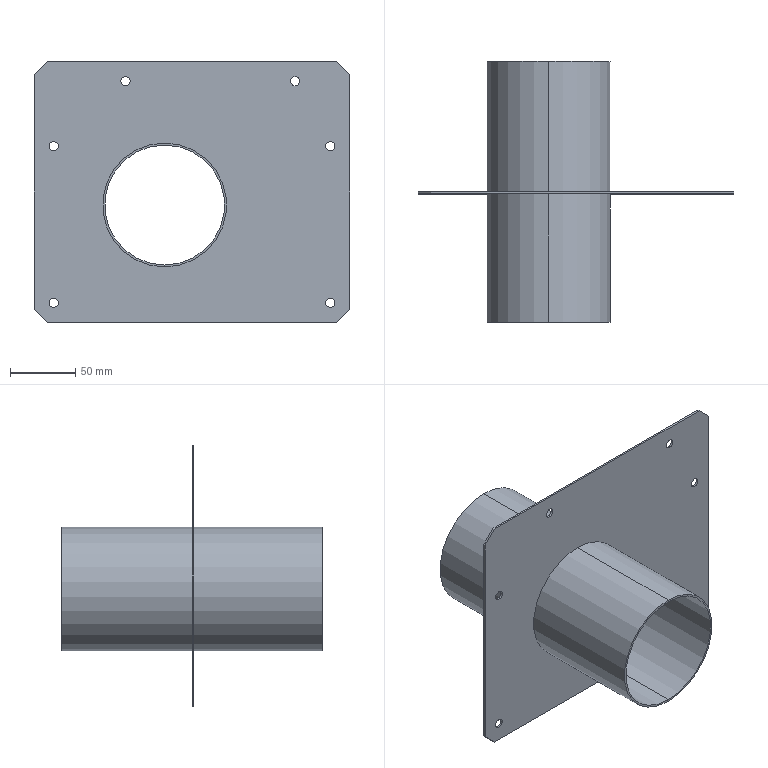Part | SolidWorks | features BaseBody 1 | 1 solid | 30 faces | box 242 x 200 x 200 mm | volume 149443 mm3 | cylinder 18 | plane 12 | commonest cylinder face diameters 7 x12 95 x4 92 x2
STEP:
#1=CARTESIAN_POINT('',(-51.,0.,88.5));
#2=VERTEX_POINT('',#1);
#3=CARTESIAN_POINT('',(-51.,0.,81.5));
#4=VERTEX_POINT('',#3);
#5=CARTESIAN_POINT('',(-51.,0.,85.));
#6=DIRECTION('',(0.,-1.,0.));
#7=DIRECTION('',(0.,0.,1.));
#8=AXIS2_PLACEMENT_3D('',#5,#6,#7);
#9=CIRCLE('',#8,3.5);
#10=EDGE_CURVE('',#2,#4,#9,.T.);
#11=ORIENTED_EDGE('',*,*,#10,.T.);
#12=CARTESIAN_POINT('',(-51.,1.5,81.5));
#13=VERTEX_POINT('',#12);
#14=CARTESIAN_POINT('',(-51.,-98.501,81.5));
#15=DIRECTION('',(0.,1.,0.));
#16=VECTOR('',#15,1000.);
#17=LINE('',#14,#16);
#18=EDGE_CURVE('',#4,#13,#17,.T.);
#19=ORIENTED_EDGE('',*,*,#18,.T.);
#20=CARTESIAN_POINT('',(-51.,1.5,88.5));
#21=VERTEX_POINT('',#20);
#22=CARTESIAN_POINT('',(-51.,1.5,85.));
#23=DIRECTION('',(0.,1.,0.));
#24=DIRECTION('',(0.,0.,1.));
#25=AXIS2_PLACEMENT_3D('',#22,#23,#24);
#26=CIRCLE('',#25,3.5);
#27=EDGE_CURVE('',#13,#21,#26,.T.);
#28=ORIENTED_EDGE('',*,*,#27,.T.);
#29=CARTESIAN_POINT('',(-51.,-98.501,88.5));
#30=DIRECTION('',(0.,1.,0.));
#31=VECTOR('',#30,1000.);
#32=LINE('',#29,#31);
#33=EDGE_CURVE('',#2,#21,#32,.T.);
#34=ORIENTED_EDGE('',*,*,#33,.F.);
#35=EDGE_LOOP('',(#11,#19,#28,#34));
#36=FACE_OUTER_BOUND('',#35,.T.);
#37=CARTESIAN_POINT('',(-51.,-98.501,85.));
#38=DIRECTION('',(0.,1.,0.));
#39=DIRECTION('',(0.,0.,1.));
#40=AXIS2_PLACEMENT_3D('',#37,#38,#39);
#41=CYLINDRICAL_SURFACE('',#40,3.5);
#42=ADVANCED_FACE('',(#36),#41,.F.);
#43=CARTESIAN_POINT('',(79.,0.,88.5));
#44=VERTEX_POINT('',#43);
#45=CARTESIAN_POINT('',(79.,0.,81.5));
#46=VERTEX_POINT('',#45);
#47=CARTESIAN_POINT('',(79.,0.,85.));
#48=DIRECTION('',(0.,-1.,0.));
#49=DIRECTION('',(0.,0.,1.));
#50=AXIS2_PLACEMENT_3D('',#47,#48,#49);
#51=CIRCLE('',#50,3.5);
#52=EDGE_CURVE('',#44,#46,#51,.T.);
#53=ORIENTED_EDGE('',*,*,#52,.T.);
#54=CARTESIAN_POINT('',(79.,1.5,81.5));
#55=VERTEX_POINT('',#54);
#56=CARTESIAN_POINT('',(79.,-98.501,81.5));
#57=DIRECTION('',(0.,1.,0.));
#58=VECTOR('',#57,1000.);
#59=LINE('',#56,#58);
#60=EDGE_CURVE('',#46,#55,#59,.T.);
#61=ORIENTED_EDGE('',*,*,#60,.T.);
#62=CARTESIAN_POINT('',(79.,1.5,88.5));
#63=VERTEX_POINT('',#62);
#64=CARTESIAN_POINT('',(79.,1.5,85.));
#65=DIRECTION('',(0.,1.,0.));
#66=DIRECTION('',(0.,0.,1.));
#67=AXIS2_PLACEMENT_3D('',#64,#65,#66);
#68=CIRCLE('',#67,3.5);
#69=EDGE_CURVE('',#55,#63,#68,.T.);
#70=ORIENTED_EDGE('',*,*,#69,.T.);
#71=CARTESIAN_POINT('',(79.,-98.501,88.5));
#72=DIRECTION('',(0.,1.,0.));
#73=VECTOR('',#72,1000.);
#74=LINE('',#71,#73);
#75=EDGE_CURVE('',#44,#63,#74,.T.);
#76=ORIENTED_EDGE('',*,*,#75,.F.);
#77=EDGE_LOOP('',(#53,#61,#70,#76));
#78=FACE_OUTER_BOUND('',#77,.T.);
#79=CARTESIAN_POINT('',(79.,-98.501,85.));
#80=DIRECTION('',(0.,1.,0.));
#81=DIRECTION('',(0.,0.,1.));
#82=AXIS2_PLACEMENT_3D('',#79,#80,#81);
#83=CYLINDRICAL_SURFACE('',#82,3.5);
#84=ADVANCED_FACE('',(#78),#83,.F.);
#85=CARTESIAN_POINT('',(-106.,0.,38.5));
#86=VERTEX_POINT('',#85);
#87=CARTESIAN_POINT('',(-106.,0.,31.5));
#88=VERTEX_POINT('',#87);
#89=CARTESIAN_POINT('',(-106.,0.,35.));
#90=DIRECTION('',(0.,-1.,0.));
#91=DIRECTION('',(0.,0.,1.));
#92=AXIS2_PLACEMENT_3D('',#89,#90,#91);
#93=CIRCLE('',#92,3.5);
#94=EDGE_CURVE('',#86,#88,#93,.T.);
#95=ORIENTED_EDGE('',*,*,#94,.T.);
#96=CARTESIAN_POINT('',(-106.,1.5,31.5));
#97=VERTEX_POINT('',#96);
#98=CARTESIAN_POINT('',(-106.,-98.501,31.5));
#99=DIRECTION('',(0.,1.,0.));
#100=VECTOR('',#99,1000.);
#101=LINE('',#98,#100);
#102=EDGE_CURVE('',#88,#97,#101,.T.);
#103=ORIENTED_EDGE('',*,*,#102,.T.);
#104=CARTESIAN_POINT('',(-106.,1.5,38.5));
#105=VERTEX_POINT('',#104);
#106=CARTESIAN_POINT('',(-106.,1.5,35.));
#107=DIRECTION('',(0.,1.,0.));
#108=DIRECTION('',(0.,0.,1.));
#109=AXIS2_PLACEMENT_3D('',#106,#107,#108);
#110=CIRCLE('',#109,3.5);
#111=EDGE_CURVE('',#97,#105,#110,.T.);
#112=ORIENTED_EDGE('',*,*,#111,.T.);
#113=CARTESIAN_POINT('',(-106.,-98.501,38.5));
#114=DIRECTION('',(0.,1.,0.));
#115=VECTOR('',#114,1000.);
#116=LINE('',#113,#115);
#117=EDGE_CURVE('',#86,#105,#116,.T.);
#118=ORIENTED_EDGE('',*,*,#117,.F.);
#119=EDGE_LOOP('',(#95,#103,#112,#118));
#120=FACE_OUTER_BOUND('',#119,.T.);
#121=CARTESIAN_POINT('',(-106.,-98.501,35.));
#122=DIRECTION('',(0.,1.,0.));
#123=DIRECTION('',(0.,0.,1.));
#124=AXIS2_PLACEMENT_3D('',#121,#122,#123);
#125=CYLINDRICAL_SURFACE('',#124,3.5);
#126=ADVANCED_FACE('',(#120),#125,.F.);
#127=CARTESIAN_POINT('',(106.,0.,38.5));
#128=VERTEX_POINT('',#127);
#129=CARTESIAN_POINT('',(106.,0.,31.5));
#130=VERTEX_POINT('',#129);
#131=CARTESIAN_POINT('',(106.,0.,35.));
#132=DIRECTION('',(0.,-1.,0.));
#133=DIRECTION('',(0.,0.,1.));
#134=AXIS2_PLACEMENT_3D('',#131,#132,#133);
#135=CIRCLE('',#134,3.5);
#136=EDGE_CURVE('',#128,#130,#135,.T.);
#137=ORIENTED_EDGE('',*,*,#136,.T.);
#138=CARTESIAN_POINT('',(106.,1.5,31.5));
#139=VERTEX_POINT('',#138);
#140=CARTESIAN_POINT('',(106.,-98.501,31.5));
#141=DIRECTION('',(0.,1.,0.));
#142=VECTOR('',#141,1000.);
#143=LINE('',#140,#142);
#144=EDGE_CURVE('',#130,#139,#143,.T.);
#145=ORIENTED_EDGE('',*,*,#144,.T.);
#146=CARTESIAN_POINT('',(106.,1.5,38.5));
#147=VERTEX_POINT('',#146);
#148=CARTESIAN_POINT('',(106.,1.5,35.));
#149=DIRECTION('',(0.,1.,0.));
#150=DIRECTION('',(0.,0.,1.));
#151=AXIS2_PLACEMENT_3D('',#148,#149,#150);
#152=CIRCLE('',#151,3.5);
#153=EDGE_CURVE('',#139,#147,#152,.T.);
#154=ORIENTED_EDGE('',*,*,#153,.T.);
#155=CARTESIAN_POINT('',(106.,-98.501,38.5));
#156=DIRECTION('',(0.,1.,0.));
#157=VECTOR('',#156,1000.);
#158=LINE('',#155,#157);
#159=EDGE_CURVE('',#128,#147,#158,.T.);
#160=ORIENTED_EDGE('',*,*,#159,.F.);
#161=EDGE_LOOP('',(#137,#145,#154,#160));
#162=FACE_OUTER_BOUND('',#161,.T.);
#163=CARTESIAN_POINT('',(106.,-98.501,35.));
#164=DIRECTION('',(0.,1.,0.));
#165=DIRECTION('',(0.,0.,1.));
#166=AXIS2_PLACEMENT_3D('',#163,#164,#165);
#167=CYLINDRICAL_SURFACE('',#166,3.5);
#168=ADVANCED_FACE('',(#162),#167,.F.);
#169=CARTESIAN_POINT('',(-106.,0.,-81.5));
#170=VERTEX_POINT('',#169);
#171=CARTESIAN_POINT('',(-106.,0.,-88.5));
#172=VERTEX_POINT('',#171);
#173=CARTESIAN_POINT('',(-106.,0.,-85.));
#174=DIRECTION('',(0.,-1.,0.));
#175=DIRECTION('',(0.,0.,1.));
#176=AXIS2_PLACEMENT_3D('',#173,#174,#175);
#177=CIRCLE('',#176,3.5);
#178=EDGE_CURVE('',#170,#172,#177,.T.);
#179=ORIENTED_EDGE('',*,*,#178,.T.);
#180=CARTESIAN_POINT('',(-106.,1.5,-88.5));
#181=VERTEX_POINT('',#180);
#182=CARTESIAN_POINT('',(-106.,-98.501,-88.5));
#183=DIRECTION('',(0.,1.,0.));
#184=VECTOR('',#183,1000.);
#185=LINE('',#182,#184);
#186=EDGE_CURVE('',#172,#181,#185,.T.);
#187=ORIENTED_EDGE('',*,*,#186,.T.);
#188=CARTESIAN_POINT('',(-106.,1.5,-81.5));
#189=VERTEX_POINT('',#188);
#190=CARTESIAN_POINT('',(-106.,1.5,-85.));
#191=DIRECTION('',(0.,1.,0.));
#192=DIRECTION('',(0.,0.,1.));
#193=AXIS2_PLACEMENT_3D('',#190,#191,#192);
#194=CIRCLE('',#193,3.5);
#195=EDGE_CURVE('',#181,#189,#194,.T.);
#196=ORIENTED_EDGE('',*,*,#195,.T.);
#197=CARTESIAN_POINT('',(-106.,-98.501,-81.5));
#198=DIRECTION('',(0.,1.,0.));
#199=VECTOR('',#198,1000.);
#200=LINE('',#197,#199);
#201=EDGE_CURVE('',#170,#189,#200,.T.);
#202=ORIENTED_EDGE('',*,*,#201,.F.);
#203=EDGE_LOOP('',(#179,#187,#196,#202));
#204=FACE_OUTER_BOUND('',#203,.T.);
#205=CARTESIAN_POINT('',(-106.,-98.501,-85.));
#206=DIRECTION('',(0.,1.,0.));
#207=DIRECTION('',(0.,0.,1.));
#208=AXIS2_PLACEMENT_3D('',#205,#206,#207);
#209=CYLINDRICAL_SURFACE('',#208,3.5);
#210=ADVANCED_FACE('',(#204),#209,.F.);
#211=CARTESIAN_POINT('',(106.,0.,-81.5));
#212=VERTEX_POINT('',#211);
#213=CARTESIAN_POINT('',(106.,0.,-88.5));
#214=VERTEX_POINT('',#213);
#215=CARTESIAN_POINT('',(106.,0.,-85.));
#216=DIRECTION('',(0.,-1.,0.));
#217=DIRECTION('',(0.,0.,1.));
#218=AXIS2_PLACEMENT_3D('',#215,#216,#217);
#219=CIRCLE('',#218,3.5);
#220=EDGE_CURVE('',#212,#214,#219,.T.);
#221=ORIENTED_EDGE('',*,*,#220,.T.);
#222=CARTESIAN_POINT('',(106.,1.5,-88.5));
#223=VERTEX_POINT('',#222);
#224=CARTESIAN_POINT('',(106.,-98.501,-88.5));
#225=DIRECTION('',(0.,1.,0.));
#226=VECTOR('',#225,1000.);
#227=LINE('',#224,#226);
#228=EDGE_CURVE('',#214,#223,#227,.T.);
#229=ORIENTED_EDGE('',*,*,#228,.T.);
#230=CARTESIAN_POINT('',(106.,1.5,-81.5));
#231=VERTEX_POINT('',#230);
#232=CARTESIAN_POINT('',(106.,1.5,-85.));
#233=DIRECTION('',(0.,1.,0.));
#234=DIRECTION('',(0.,0.,1.));
#235=AXIS2_PLACEMENT_3D('',#232,#233,#234);
#236=CIRCLE('',#235,3.5);
#237=EDGE_CURVE('',#223,#231,#236,.T.);
#238=ORIENTED_EDGE('',*,*,#237,.T.);
#239=CARTESIAN_POINT('',(106.,-98.501,-81.5));
#240=DIRECTION('',(0.,1.,0.));
#241=VECTOR('',#240,1000.);
#242=LINE('',#239,#241);
#243=EDGE_CURVE('',#212,#231,#242,.T.);
#244=ORIENTED_EDGE('',*,*,#243,.F.);
#245=EDGE_LOOP('',(#221,#229,#238,#244));
#246=FACE_OUTER_BOUND('',#245,.T.);
#247=CARTESIAN_POINT('',(106.,-98.501,-85.));
#248=DIRECTION('',(0.,1.,0.));
#249=DIRECTION('',(0.,0.,1.));
#250=AXIS2_PLACEMENT_3D('',#247,#248,#249);
#251=CYLINDRICAL_SURFACE('',#250,3.5);
#252=ADVANCED_FACE('',(#246),#251,.F.);
#253=CARTESIAN_POINT('',(-21.,101.5,37.5));
#254=VERTEX_POINT('',#253);
#255=CARTESIAN_POINT('',(-21.,101.5,-57.5));
#256=VERTEX_POINT('',#255);
#257=CARTESIAN_POINT('',(-21.,101.5,-10.));
#258=DIRECTION('',(0.,1.,0.));
#259=DIRECTION('',(0.,0.,1.));
#260=AXIS2_PLACEMENT_3D('',#257,#258,#259);
#261=CIRCLE('',#260,47.5);
#262=EDGE_CURVE('',#254,#256,#261,.T.);
#263=ORIENTED_EDGE('',*,*,#262,.F.);
#264=CARTESIAN_POINT('',(-21.,1.5,37.5));
#265=VERTEX_POINT('',#264);
#266=CARTESIAN_POINT('',(-21.,101.5,37.5));
#267=DIRECTION('',(0.,-1.,0.));
#268=VECTOR('',#267,1000.);
#269=LINE('',#266,#268);
#270=EDGE_CURVE('',#254,#265,#269,.T.);
#271=ORIENTED_EDGE('',*,*,#270,.T.);
#272=CARTESIAN_POINT('',(-21.,1.5,-57.5));
#273=VERTEX_POINT('',#272);
#274=CARTESIAN_POINT('',(-21.,1.5,-10.));
#275=DIRECTION('',(0.,1.,0.));
#276=DIRECTION('',(0.,0.,1.));
#277=AXIS2_PLACEMENT_3D('',#274,#275,#276);
#278=CIRCLE('',#277,47.5);
#279=EDGE_CURVE('',#265,#273,#278,.T.);
#280=ORIENTED_EDGE('',*,*,#279,.T.);
#281=CARTESIAN_POINT('',(-21.,101.5,-57.5));
#282=DIRECTION('',(0.,-1.,0.));
#283=VECTOR('',#282,1000.);
#284=LINE('',#281,#283);
#285=EDGE_CURVE('',#256,#273,#284,.T.);
#286=ORIENTED_EDGE('',*,*,#285,.F.);
#287=EDGE_LOOP('',(#263,#271,#280,#286));
#288=FACE_OUTER_BOUND('',#287,.T.);
#289=CARTESIAN_POINT('',(-21.,101.5,-10.));
#290=DIRECTION('',(0.,-1.,0.));
#291=DIRECTION('',(0.,0.,-1.));
#292=AXIS2_PLACEMENT_3D('',#289,#290,#291);
#293=CYLINDRICAL_SURFACE('',#292,47.5);
#294=ADVANCED_FACE('',(#288),#293,.T.);
#295=CARTESIAN_POINT('',(-21.,-98.5,-57.5));
#296=VERTEX_POINT('',#295);
#297=CARTESIAN_POINT('',(-21.,-98.5,37.5));
#298=VERTEX_POINT('',#297);
#299=CARTESIAN_POINT('',(-21.,-98.5,-10.));
#300=DIRECTION('',(0.,-1.,0.));
#301=DIRECTION('',(0.,0.,-1.));
#302=AXIS2_PLACEMENT_3D('',#299,#300,#301);
#303=CIRCLE('',#302,47.5);
#304=EDGE_CURVE('',#296,#298,#303,.T.);
#305=ORIENTED_EDGE('',*,*,#304,.F.);
#306=CARTESIAN_POINT('',(-21.,0.,-57.5));
#307=VERTEX_POINT('',#306);
#308=CARTESIAN_POINT('',(-21.,-98.5,-57.5));
#309=DIRECTION('',(0.,1.,0.));
#310=VECTOR('',#309,1000.);
#311=LINE('',#308,#310);
#312=EDGE_CURVE('',#296,#307,#311,.T.);
#313=ORIENTED_EDGE('',*,*,#312,.T.);
#314=CARTESIAN_POINT('',(-21.,0.,37.5));
#315=VERTEX_POINT('',#314);
#316=CARTESIAN_POINT('',(-21.,0.,-10.));
#317=DIRECTION('',(0.,-1.,0.));
#318=DIRECTION('',(0.,0.,1.));
#319=AXIS2_PLACEMENT_3D('',#316,#317,#318);
#320=CIRCLE('',#319,47.5);
#321=EDGE_CURVE('',#307,#315,#320,.T.);
#322=ORIENTED_EDGE('',*,*,#321,.T.);
#323=CARTESIAN_POINT('',(-21.,-98.5,37.5));
#324=DIRECTION('',(0.,1.,0.));
#325=VECTOR('',#324,1000.);
#326=LINE('',#323,#325);
#327=EDGE_CURVE('',#298,#315,#326,.T.);
#328=ORIENTED_EDGE('',*,*,#327,.F.);
#329=EDGE_LOOP('',(#305,#313,#322,#328));
#330=FACE_OUTER_BOUND('',#329,.T.);
#331=CARTESIAN_POINT('',(-21.,-98.5,-10.));
#332=DIRECTION('',(0.,1.,0.));
#333=DIRECTION('',(0.,0.,1.));
#334=AXIS2_PLACEMENT_3D('',#331,#332,#333);
#335=CYLINDRICAL_SURFACE('',#334,47.5);
#336=ADVANCED_FACE('',(#330),#335,.T.);
#337=CARTESIAN_POINT('',(-21.,-98.5,36.));
#338=VERTEX_POINT('',#337);
#339=CARTESIAN_POINT('',(-21.,-98.5,-56.));
#340=VERTEX_POINT('',#339);
#341=CARTESIAN_POINT('',(-21.,-98.5,-10.));
#342=DIRECTION('',(0.,-1.,0.));
#343=DIRECTION('',(0.,0.,-1.));
#344=AXIS2_PLACEMENT_3D('',#341,#342,#343);
#345=CIRCLE('',#344,46.);
#346=EDGE_CURVE('',#338,#340,#345,.T.);
#347=ORIENTED_EDGE('',*,*,#346,.T.);
#348=CARTESIAN_POINT('',(-21.,101.5,-56.));
#349=VERTEX_POINT('',#348);
#350=CARTESIAN_POINT('',(-21.,-0.5,-56.));
#351=DIRECTION('',(0.,1.,0.));
#352=VECTOR('',#351,1000.);
#353=LINE('',#350,#352);
#354=EDGE_CURVE('',#340,#349,#353,.T.);
#355=ORIENTED_EDGE('',*,*,#354,.T.);
#356=CARTESIAN_POINT('',(-21.,101.5,36.));
#357=VERTEX_POINT('',#356);
#358=CARTESIAN_POINT('',(-21.,101.5,-10.));
#359=DIRECTION('',(0.,1.,0.));
#360=DIRECTION('',(0.,0.,1.));
#361=AXIS2_PLACEMENT_3D('',#358,#359,#360);
#362=CIRCLE('',#361,46.);
#363=EDGE_CURVE('',#349,#357,#362,.T.);
#364=ORIENTED_EDGE('',*,*,#363,.T.);
#365=CARTESIAN_POINT('',(-21.,-0.5,36.));
#366=DIRECTION('',(0.,1.,0.));
#367=VECTOR('',#366,1000.);
#368=LINE('',#365,#367);
#369=EDGE_CURVE('',#338,#357,#368,.T.);
#370=ORIENTED_EDGE('',*,*,#369,.F.);
#371=EDGE_LOOP('',(#347,#355,#364,#370));
#372=FACE_OUTER_BOUND('',#371,.T.);
#373=CARTESIAN_POINT('',(-21.,-0.5,-10.));
#374=DIRECTION('',(0.,1.,0.));
#375=DIRECTION('',(0.,0.,1.));
#376=AXIS2_PLACEMENT_3D('',#373,#374,#375);
#377=CYLINDRICAL_SURFACE('',#376,46.);
#378=ADVANCED_FACE('',(#372),#377,.F.);
#379=CARTESIAN_POINT('',(-21.,101.5,-10.));
#380=DIRECTION('',(0.,1.,0.));
#381=DIRECTION('',(0.,0.,1.));
#382=AXIS2_PLACEMENT_3D('',#379,#380,#381);
#383=CIRCLE('',#382,46.);
#384=EDGE_CURVE('',#357,#349,#383,.T.);
#385=ORIENTED_EDGE('',*,*,#384,.F.);
#386=ORIENTED_EDGE('',*,*,#363,.F.);
#387=EDGE_LOOP('',(#385,#386));
#388=FACE_BOUND('',#387,.T.);
#389=CARTESIAN_POINT('',(-21.,101.5,-10.));
#390=DIRECTION('',(0.,1.,0.));
#391=DIRECTION('',(0.,0.,1.));
#392=AXIS2_PLACEMENT_3D('',#389,#390,#391);
#393=CIRCLE('',#392,47.5);
#394=EDGE_CURVE('',#256,#254,#393,.T.);
#395=ORIENTED_EDGE('',*,*,#394,.T.);
#396=ORIENTED_EDGE('',*,*,#262,.T.);
#397=EDGE_LOOP('',(#395,#396));
#398=FACE_OUTER_BOUND('',#397,.T.);
#399=CARTESIAN_POINT('',(-21.,101.5,-10.));
#400=DIRECTION('',(0.,1.,0.));
#401=DIRECTION('',(1.,0.,0.));
#402=AXIS2_PLACEMENT_3D('',#399,#400,#401);
#403=PLANE('',#402);
#404=ADVANCED_FACE('',(#388,#398),#403,.T.);
#405=ORIENTED_EDGE('',*,*,#346,.F.);
#406=CARTESIAN_POINT('',(-21.,-98.5,-10.));
#407=DIRECTION('',(0.,-1.,0.));
#408=DIRECTION('',(0.,0.,-1.));
#409=AXIS2_PLACEMENT_3D('',#406,#407,#408);
#410=CIRCLE('',#409,46.);
#411=EDGE_CURVE('',#340,#338,#410,.T.);
#412=ORIENTED_EDGE('',*,*,#411,.F.);
#413=EDGE_LOOP('',(#405,#412));
#414=FACE_BOUND('',#413,.T.);
#415=CARTESIAN_POINT('',(-21.,-98.5,-10.));
#416=DIRECTION('',(0.,-1.,0.));
#417=DIRECTION('',(0.,0.,-1.));
#418=AXIS2_PLACEMENT_3D('',#415,#416,#417);
#419=CIRCLE('',#418,47.5);
#420=EDGE_CURVE('',#298,#296,#419,.T.);
#421=ORIENTED_EDGE('',*,*,#420,.T.);
#422=ORIENTED_EDGE('',*,*,#304,.T.);
#423=EDGE_LOOP('',(#421,#422));
#424=FACE_OUTER_BOUND('',#423,.T.);
#425=CARTESIAN_POINT('',(-21.,-98.5,-10.));
#426=DIRECTION('',(0.,-1.,0.));
#427=DIRECTION('',(0.,0.,-1.));
#428=AXIS2_PLACEMENT_3D('',#425,#426,#427);
#429=PLANE('',#428);
#430=ADVANCED_FACE('',(#414,#424),#429,.T.);
#431=CARTESIAN_POINT('',(-121.,1.5,90.));
#432=VERTEX_POINT('',#431);
#433=CARTESIAN_POINT('',(-111.,1.5,100.));
#434=VERTEX_POINT('',#433);
#435=CARTESIAN_POINT('',(-105.5,1.5,105.5));
#436=DIRECTION('',(0.7071,0.,0.7071));
#437=VECTOR('',#436,1000.);
#438=LINE('',#435,#437);
#439=EDGE_CURVE('',#432,#434,#438,.T.);
#440=ORIENTED_EDGE('',*,*,#439,.F.);
#441=CARTESIAN_POINT('',(-121.,0.,90.));
#442=VERTEX_POINT('',#441);
#443=CARTESIAN_POINT('',(-121.,1.5,90.));
#444=DIRECTION('',(0.,1.,0.));
#445=VECTOR('',#444,1000.);
#446=LINE('',#443,#445);
#447=EDGE_CURVE('',#442,#432,#446,.T.);
#448=ORIENTED_EDGE('',*,*,#447,.F.);
#449=CARTESIAN_POINT('',(-111.,0.,100.));
#450=VERTEX_POINT('',#449);
#451=CARTESIAN_POINT('',(-111.,0.,100.));
#452=DIRECTION('',(-0.7071,0.,-0.7071));
#453=VECTOR('',#452,1000.);
#454=LINE('',#451,#453);
#455=EDGE_CURVE('',#450,#442,#454,.T.);
#456=ORIENTED_EDGE('',*,*,#455,.F.);
#457=CARTESIAN_POINT('',(-111.,1.5,100.));
#458=DIRECTION('',(0.,-1.,0.));
#459=VECTOR('',#458,1000.);
#460=LINE('',#457,#459);
#461=EDGE_CURVE('',#434,#450,#460,.T.);
#462=ORIENTED_EDGE('',*,*,#461,.F.);
#463=EDGE_LOOP('',(#440,#448,#456,#462));
#464=FACE_OUTER_BOUND('',#463,.T.);
#465=CARTESIAN_POINT('',(-111.,1.5,100.));
#466=DIRECTION('',(0.7071,0.,-0.7071));
#467=DIRECTION('',(0.,-1.,0.));
#468=AXIS2_PLACEMENT_3D('',#465,#466,#467);
#469=PLANE('',#468);
#470=ADVANCED_FACE('',(#464),#469,.F.);
#471=CARTESIAN_POINT('',(-111.,1.5,-100.));
#472=VERTEX_POINT('',#471);
#473=CARTESIAN_POINT('',(-121.,1.5,-90.));
#474=VERTEX_POINT('',#473);
#475=CARTESIAN_POINT('',(-105.5,1.5,-105.5));
#476=DIRECTION('',(-0.7071,0.,0.7071));
#477=VECTOR('',#476,1000.);
#478=LINE('',#475,#477);
#479=EDGE_CURVE('',#472,#474,#478,.T.);
#480=ORIENTED_EDGE('',*,*,#479,.F.);
#481=CARTESIAN_POINT('',(-111.,0.,-100.));
#482=VERTEX_POINT('',#481);
#483=CARTESIAN_POINT('',(-111.,1.5,-100.));
#484=DIRECTION('',(0.,1.,0.));
#485=VECTOR('',#484,1000.);
#486=LINE('',#483,#485);
#487=EDGE_CURVE('',#482,#472,#486,.T.);
#488=ORIENTED_EDGE('',*,*,#487,.F.);
#489=CARTESIAN_POINT('',(-121.,0.,-90.));
#490=VERTEX_POINT('',#489);
#491=CARTESIAN_POINT('',(-121.,0.,-90.));
#492=DIRECTION('',(0.7071,0.,-0.7071));
#493=VECTOR('',#492,1000.);
#494=LINE('',#491,#493);
#495=EDGE_CURVE('',#490,#482,#494,.T.);
#496=ORIENTED_EDGE('',*,*,#495,.F.);
#497=CARTESIAN_POINT('',(-121.,1.5,-90.));
#498=DIRECTION('',(0.,-1.,0.));
#499=VECTOR('',#498,1000.);
#500=LINE('',#497,#499);
#501=EDGE_CURVE('',#474,#490,#500,.T.);
#502=ORIENTED_EDGE('',*,*,#501,.F.);
#503=EDGE_LOOP('',(#480,#488,#496,#502));
#504=FACE_OUTER_BOUND('',#503,.T.);
#505=CARTESIAN_POINT('',(-121.,1.5,-90.));
#506=DIRECTION('',(0.7071,0.,0.7071));
#507=DIRECTION('',(0.,-1.,0.));
#508=AXIS2_PLACEMENT_3D('',#505,#506,#507);
#509=PLANE('',#508);
#510=ADVANCED_FACE('',(#504),#509,.F.);
#511=CARTESIAN_POINT('',(121.,1.5,-90.));
#512=VERTEX_POINT('',#511);
#513=CARTESIAN_POINT('',(111.,1.5,-100.));
#514=VERTEX_POINT('',#513);
#515=CARTESIAN_POINT('',(105.5,1.5,-105.5));
#516=DIRECTION('',(-0.7071,0.,-0.7071));
#517=VECTOR('',#516,1000.);
#518=LINE('',#515,#517);
#519=EDGE_CURVE('',#512,#514,#518,.T.);
#520=ORIENTED_EDGE('',*,*,#519,.F.);
#521=CARTESIAN_POINT('',(121.,0.,-90.));
#522=VERTEX_POINT('',#521);
#523=CARTESIAN_POINT('',(121.,1.5,-90.));
#524=DIRECTION('',(0.,1.,0.));
#525=VECTOR('',#524,1000.);
#526=LINE('',#523,#525);
#527=EDGE_CURVE('',#522,#512,#526,.T.);
#528=ORIENTED_EDGE('',*,*,#527,.F.);
#529=CARTESIAN_POINT('',(111.,0.,-100.));
#530=VERTEX_POINT('',#529);
#531=CARTESIAN_POINT('',(111.,0.,-100.));
#532=DIRECTION('',(0.7071,0.,0.7071));
#533=VECTOR('',#532,1000.);
#534=LINE('',#531,#533);
#535=EDGE_CURVE('',#530,#522,#534,.T.);
#536=ORIENTED_EDGE('',*,*,#535,.F.);
#537=CARTESIAN_POINT('',(111.,1.5,-100.));
#538=DIRECTION('',(0.,-1.,0.));
#539=VECTOR('',#538,1000.);
#540=LINE('',#537,#539);
#541=EDGE_CURVE('',#514,#530,#540,.T.);
#542=ORIENTED_EDGE('',*,*,#541,.F.);
#543=EDGE_LOOP('',(#520,#528,#536,#542));
#544=FACE_OUTER_BOUND('',#543,.T.);
#545=CARTESIAN_POINT('',(111.,1.5,-100.));
#546=DIRECTION('',(-0.7071,0.,0.7071));
#547=DIRECTION('',(0.,1.,0.));
#548=AXIS2_PLACEMENT_3D('',#545,#546,#547);
#549=PLANE('',#548);
#550=ADVANCED_FACE('',(#544),#549,.F.);
#551=CARTESIAN_POINT('',(111.,1.5,100.));
#552=VERTEX_POINT('',#551);
#553=CARTESIAN_POINT('',(121.,1.5,90.));
#554=VERTEX_POINT('',#553);
#555=CARTESIAN_POINT('',(105.5,1.5,105.5));
#556=DIRECTION('',(0.7071,0.,-0.7071));
#557=VECTOR('',#556,1000.);
#558=LINE('',#555,#557);
#559=EDGE_CURVE('',#552,#554,#558,.T.);
#560=ORIENTED_EDGE('',*,*,#559,.F.);
#561=CARTESIAN_POINT('',(111.,0.,100.));
#562=VERTEX_POINT('',#561);
#563=CARTESIAN_POINT('',(111.,1.5,100.));
#564=DIRECTION('',(0.,1.,0.));
#565=VECTOR('',#564,1000.);
#566=LINE('',#563,#565);
#567=EDGE_CURVE('',#562,#552,#566,.T.);
#568=ORIENTED_EDGE('',*,*,#567,.F.);
#569=CARTESIAN_POINT('',(121.,0.,90.));
#570=VERTEX_POINT('',#569);
#571=CARTESIAN_POINT('',(121.,0.,90.));
#572=DIRECTION('',(-0.7071,0.,0.7071));
#573=VECTOR('',#572,1000.);
#574=LINE('',#571,#573);
#575=EDGE_CURVE('',#570,#562,#574,.T.);
#576=ORIENTED_EDGE('',*,*,#575,.F.);
#577=CARTESIAN_POINT('',(121.,1.5,90.));
#578=DIRECTION('',(0.,-1.,0.));
#579=VECTOR('',#578,1000.);
#580=LINE('',#577,#579);
#581=EDGE_CURVE('',#554,#570,#580,.T.);
#582=ORIENTED_EDGE('',*,*,#581,.F.);
#583=EDGE_LOOP('',(#560,#568,#576,#582));
#584=FACE_OUTER_BOUND('',#583,.T.);
#585=CARTESIAN_POINT('',(121.,1.5,90.));
#586=DIRECTION('',(-0.7071,0.,-0.7071));
#587=DIRECTION('',(-0.7071,0.,0.7071));
#588=AXIS2_PLACEMENT_3D('',#585,#586,#587);
#589=PLANE('',#588);
#590=ADVANCED_FACE('',(#584),#589,.F.);
#591=CARTESIAN_POINT('',(-121.,0.,100.));
#592=DIRECTION('',(1.,0.,0.));
#593=VECTOR('',#592,1000.);
#594=LINE('',#591,#593);
#595=EDGE_CURVE('',#450,#562,#594,.T.);
#596=ORIENTED_EDGE('',*,*,#595,.T.);
#597=ORIENTED_EDGE('',*,*,#567,.T.);
#598=CARTESIAN_POINT('',(-121.,1.5,100.));
#599=DIRECTION('',(1.,0.,0.));
#600=VECTOR('',#599,1000.);
#601=LINE('',#598,#600);
#602=EDGE_CURVE('',#434,#552,#601,.T.);
#603=ORIENTED_EDGE('',*,*,#602,.F.);
#604=ORIENTED_EDGE('',*,*,#461,.T.);
#605=EDGE_LOOP('',(#596,#597,#603,#604));
#606=FACE_OUTER_BOUND('',#605,.T.);
#607=CARTESIAN_POINT('',(-121.,1.5,100.));
#608=DIRECTION('',(0.,0.,-1.));
#609=DIRECTION('',(0.,-1.,0.));
#610=AXIS2_PLACEMENT_3D('',#607,#608,#609);
#611=PLANE('',#610);
#612=ADVANCED_FACE('',(#606),#611,.F.);
#613=CARTESIAN_POINT('',(-121.,1.5,-100.));
#614=DIRECTION('',(0.,0.,1.));
#615=VECTOR('',#614,1000.);
#616=LINE('',#613,#615);
#617=EDGE_CURVE('',#474,#432,#616,.T.);
#618=ORIENTED_EDGE('',*,*,#617,.F.);
#619=ORIENTED_EDGE('',*,*,#501,.T.);
#620=CARTESIAN_POINT('',(-121.,0.,-100.));
#621=DIRECTION('',(0.,0.,1.));
#622=VECTOR('',#621,1000.);
#623=LINE('',#620,#622);
#624=EDGE_CURVE('',#490,#442,#623,.T.);
#625=ORIENTED_EDGE('',*,*,#624,.T.);
#626=ORIENTED_EDGE('',*,*,#447,.T.);
#627=EDGE_LOOP('',(#618,#619,#625,#626));
#628=FACE_OUTER_BOUND('',#627,.T.);
#629=CARTESIAN_POINT('',(-121.,1.5,-100.));
#630=DIRECTION('',(1.,0.,0.));
#631=DIRECTION('',(0.,0.,-1.));
#632=AXIS2_PLACEMENT_3D('',#629,#630,#631);
#633=PLANE('',#632);
#634=ADVANCED_FACE('',(#628),#633,.F.);
#635=CARTESIAN_POINT('',(-121.,1.5,-100.));
#636=DIRECTION('',(-1.,0.,0.));
#637=VECTOR('',#636,1000.);
#638=LINE('',#635,#637);
#639=EDGE_CURVE('',#514,#472,#638,.T.);
#640=ORIENTED_EDGE('',*,*,#639,.F.);
#641=ORIENTED_EDGE('',*,*,#541,.T.);
#642=CARTESIAN_POINT('',(-121.,0.,-100.));
#643=DIRECTION('',(-1.,0.,0.));
#644=VECTOR('',#643,1000.);
#645=LINE('',#642,#644);
#646=EDGE_CURVE('',#530,#482,#645,.T.);
#647=ORIENTED_EDGE('',*,*,#646,.T.);
#648=ORIENTED_EDGE('',*,*,#487,.T.);
#649=EDGE_LOOP('',(#640,#641,#647,#648));
#650=FACE_OUTER_BOUND('',#649,.T.);
#651=CARTESIAN_POINT('',(-121.,1.5,-100.));
#652=DIRECTION('',(0.,0.,1.));
#653=DIRECTION('',(1.,0.,0.));
#654=AXIS2_PLACEMENT_3D('',#651,#652,#653);
#655=PLANE('',#654);
#656=ADVANCED_FACE('',(#650),#655,.F.);
#657=CARTESIAN_POINT('',(121.,1.5,-100.));
#658=DIRECTION('',(0.,0.,-1.));
#659=VECTOR('',#658,1000.);
#660=LINE('',#657,#659);
#661=EDGE_CURVE('',#554,#512,#660,.T.);
#662=ORIENTED_EDGE('',*,*,#661,.F.);
#663=ORIENTED_EDGE('',*,*,#581,.T.);
#664=CARTESIAN_POINT('',(121.,0.,-100.));
#665=DIRECTION('',(0.,0.,-1.));
#666=VECTOR('',#665,1000.);
#667=LINE('',#664,#666);
#668=EDGE_CURVE('',#570,#522,#667,.T.);
#669=ORIENTED_EDGE('',*,*,#668,.T.);
#670=ORIENTED_EDGE('',*,*,#527,.T.);
#671=EDGE_LOOP('',(#662,#663,#669,#670));
#672=FACE_OUTER_BOUND('',#671,.T.);
#673=CARTESIAN_POINT('',(121.,1.5,-100.));
#674=DIRECTION('',(-1.,0.,0.));
#675=DIRECTION('',(0.,1.,0.));
#676=AXIS2_PLACEMENT_3D('',#673,#674,#675);
#677=PLANE('',#676);
#678=ADVANCED_FACE('',(#672),#677,.F.);
#679=CARTESIAN_POINT('',(-21.,0.,-10.));
#680=DIRECTION('',(0.,-1.,0.));
#681=DIRECTION('',(0.,0.,1.));
#682=AXIS2_PLACEMENT_3D('',#679,#680,#681);
#683=CIRCLE('',#682,47.5);
#684=EDGE_CURVE('',#315,#307,#683,.T.);
#685=ORIENTED_EDGE('',*,*,#684,.F.);
#686=ORIENTED_EDGE('',*,*,#321,.F.);
#687=EDGE_LOOP('',(#685,#686));
#688=FACE_BOUND('',#687,.T.);
#689=ORIENTED_EDGE('',*,*,#220,.F.);
#690=CARTESIAN_POINT('',(106.,0.,-85.));
#691=DIRECTION('',(0.,-1.,0.));
#692=DIRECTION('',(0.,0.,1.));
#693=AXIS2_PLACEMENT_3D('',#690,#691,#692);
#694=CIRCLE('',#693,3.5);
#695=EDGE_CURVE('',#214,#212,#694,.T.);
#696=ORIENTED_EDGE('',*,*,#695,.F.);
#697=EDGE_LOOP('',(#689,#696));
#698=FACE_BOUND('',#697,.T.);
#699=ORIENTED_EDGE('',*,*,#178,.F.);
#700=CARTESIAN_POINT('',(-106.,0.,-85.));
#701=DIRECTION('',(0.,-1.,0.));
#702=DIRECTION('',(0.,0.,1.));
#703=AXIS2_PLACEMENT_3D('',#700,#701,#702);
#704=CIRCLE('',#703,3.5);
#705=EDGE_CURVE('',#172,#170,#704,.T.);
#706=ORIENTED_EDGE('',*,*,#705,.F.);
#707=EDGE_LOOP('',(#699,#706));
#708=FACE_BOUND('',#707,.T.);
#709=ORIENTED_EDGE('',*,*,#136,.F.);
#710=CARTESIAN_POINT('',(106.,0.,35.));
#711=DIRECTION('',(0.,-1.,0.));
#712=DIRECTION('',(0.,0.,1.));
#713=AXIS2_PLACEMENT_3D('',#710,#711,#712);
#714=CIRCLE('',#713,3.5);
#715=EDGE_CURVE('',#130,#128,#714,.T.);
#716=ORIENTED_EDGE('',*,*,#715,.F.);
#717=EDGE_LOOP('',(#709,#716));
#718=FACE_BOUND('',#717,.T.);
#719=ORIENTED_EDGE('',*,*,#94,.F.);
#720=CARTESIAN_POINT('',(-106.,0.,35.));
#721=DIRECTION('',(0.,-1.,0.));
#722=DIRECTION('',(0.,0.,1.));
#723=AXIS2_PLACEMENT_3D('',#720,#721,#722);
#724=CIRCLE('',#723,3.5);
#725=EDGE_CURVE('',#88,#86,#724,.T.);
#726=ORIENTED_EDGE('',*,*,#725,.F.);
#727=EDGE_LOOP('',(#719,#726));
#728=FACE_BOUND('',#727,.T.);
#729=ORIENTED_EDGE('',*,*,#52,.F.);
#730=CARTESIAN_POINT('',(79.,0.,85.));
#731=DIRECTION('',(0.,-1.,0.));
#732=DIRECTION('',(0.,0.,1.));
#733=AXIS2_PLACEMENT_3D('',#730,#731,#732);
#734=CIRCLE('',#733,3.5);
#735=EDGE_CURVE('',#46,#44,#734,.T.);
#736=ORIENTED_EDGE('',*,*,#735,.F.);
#737=EDGE_LOOP('',(#729,#736));
#738=FACE_BOUND('',#737,.T.);
#739=ORIENTED_EDGE('',*,*,#10,.F.);
#740=CARTESIAN_POINT('',(-51.,0.,85.));
#741=DIRECTION('',(0.,-1.,0.));
#742=DIRECTION('',(0.,0.,1.));
#743=AXIS2_PLACEMENT_3D('',#740,#741,#742);
#744=CIRCLE('',#743,3.5);
#745=EDGE_CURVE('',#4,#2,#744,.T.);
#746=ORIENTED_EDGE('',*,*,#745,.F.);
#747=EDGE_LOOP('',(#739,#746));
#748=FACE_BOUND('',#747,.T.);
#749=ORIENTED_EDGE('',*,*,#668,.F.);
#750=ORIENTED_EDGE('',*,*,#575,.T.);
#751=ORIENTED_EDGE('',*,*,#595,.F.);
#752=ORIENTED_EDGE('',*,*,#455,.T.);
#753=ORIENTED_EDGE('',*,*,#624,.F.);
#754=ORIENTED_EDGE('',*,*,#495,.T.);
#755=ORIENTED_EDGE('',*,*,#646,.F.);
#756=ORIENTED_EDGE('',*,*,#535,.T.);
#757=EDGE_LOOP('',(#749,#750,#751,#752,#753,#754,#755,#756));
#758=FACE_OUTER_BOUND('',#757,.T.);
#759=CARTESIAN_POINT('',(0.,0.,0.));
#760=DIRECTION('',(0.,1.,0.));
#761=DIRECTION('',(1.,0.,0.));
#762=AXIS2_PLACEMENT_3D('',#759,#760,#761);
#763=PLANE('',#762);
#764=ADVANCED_FACE('',(#688,#698,#708,#718,#728,#738,#748,#758),#763,.F.);
#765=CARTESIAN_POINT('',(-21.,1.5,-10.));
#766=DIRECTION('',(0.,1.,0.));
#767=DIRECTION('',(0.,0.,1.));
#768=AXIS2_PLACEMENT_3D('',#765,#766,#767);
#769=CIRCLE('',#768,47.5);
#770=EDGE_CURVE('',#273,#265,#769,.T.);
#771=ORIENTED_EDGE('',*,*,#770,.F.);
#772=ORIENTED_EDGE('',*,*,#279,.F.);
#773=EDGE_LOOP('',(#771,#772));
#774=FACE_BOUND('',#773,.T.);
#775=CARTESIAN_POINT('',(106.,1.5,-85.));
#776=DIRECTION('',(0.,1.,0.));
#777=DIRECTION('',(0.,0.,1.));
#778=AXIS2_PLACEMENT_3D('',#775,#776,#777);
#779=CIRCLE('',#778,3.5);
#780=EDGE_CURVE('',#231,#223,#779,.T.);
#781=ORIENTED_EDGE('',*,*,#780,.F.);
#782=ORIENTED_EDGE('',*,*,#237,.F.);
#783=EDGE_LOOP('',(#781,#782));
#784=FACE_BOUND('',#783,.T.);
#785=CARTESIAN_POINT('',(-106.,1.5,-85.));
#786=DIRECTION('',(0.,1.,0.));
#787=DIRECTION('',(0.,0.,1.));
#788=AXIS2_PLACEMENT_3D('',#785,#786,#787);
#789=CIRCLE('',#788,3.5);
#790=EDGE_CURVE('',#189,#181,#789,.T.);
#791=ORIENTED_EDGE('',*,*,#790,.F.);
#792=ORIENTED_EDGE('',*,*,#195,.F.);
#793=EDGE_LOOP('',(#791,#792));
#794=FACE_BOUND('',#793,.T.);
#795=CARTESIAN_POINT('',(106.,1.5,35.));
#796=DIRECTION('',(0.,1.,0.));
#797=DIRECTION('',(0.,0.,1.));
#798=AXIS2_PLACEMENT_3D('',#795,#796,#797);
#799=CIRCLE('',#798,3.5);
#800=EDGE_CURVE('',#147,#139,#799,.T.);
#801=ORIENTED_EDGE('',*,*,#800,.F.);
#802=ORIENTED_EDGE('',*,*,#153,.F.);
#803=EDGE_LOOP('',(#801,#802));
#804=FACE_BOUND('',#803,.T.);
#805=CARTESIAN_POINT('',(-106.,1.5,35.));
#806=DIRECTION('',(0.,1.,0.));
#807=DIRECTION('',(0.,0.,1.));
#808=AXIS2_PLACEMENT_3D('',#805,#806,#807);
#809=CIRCLE('',#808,3.5);
#810=EDGE_CURVE('',#105,#97,#809,.T.);
#811=ORIENTED_EDGE('',*,*,#810,.F.);
#812=ORIENTED_EDGE('',*,*,#111,.F.);
#813=EDGE_LOOP('',(#811,#812));
#814=FACE_BOUND('',#813,.T.);
#815=CARTESIAN_POINT('',(79.,1.5,85.));
#816=DIRECTION('',(0.,1.,0.));
#817=DIRECTION('',(0.,0.,1.));
#818=AXIS2_PLACEMENT_3D('',#815,#816,#817);
#819=CIRCLE('',#818,3.5);
#820=EDGE_CURVE('',#63,#55,#819,.T.);
#821=ORIENTED_EDGE('',*,*,#820,.F.);
#822=ORIENTED_EDGE('',*,*,#69,.F.);
#823=EDGE_LOOP('',(#821,#822));
#824=FACE_BOUND('',#823,.T.);
#825=CARTESIAN_POINT('',(-51.,1.5,85.));
#826=DIRECTION('',(0.,1.,0.));
#827=DIRECTION('',(0.,0.,1.));
#828=AXIS2_PLACEMENT_3D('',#825,#826,#827);
#829=CIRCLE('',#828,3.5);
#830=EDGE_CURVE('',#21,#13,#829,.T.);
#831=ORIENTED_EDGE('',*,*,#830,.F.);
#832=ORIENTED_EDGE('',*,*,#27,.F.);
#833=EDGE_LOOP('',(#831,#832));
#834=FACE_BOUND('',#833,.T.);
#835=ORIENTED_EDGE('',*,*,#602,.T.);
#836=ORIENTED_EDGE('',*,*,#559,.T.);
#837=ORIENTED_EDGE('',*,*,#661,.T.);
#838=ORIENTED_EDGE('',*,*,#519,.T.);
#839=ORIENTED_EDGE('',*,*,#639,.T.);
#840=ORIENTED_EDGE('',*,*,#479,.T.);
#841=ORIENTED_EDGE('',*,*,#617,.T.);
#842=ORIENTED_EDGE('',*,*,#439,.T.);
#843=EDGE_LOOP('',(#835,#836,#837,#838,#839,#840,#841,#842));
#844=FACE_OUTER_BOUND('',#843,.T.);
#845=CARTESIAN_POINT('',(0.,1.5,0.));
#846=DIRECTION('',(0.,1.,0.));
#847=DIRECTION('',(1.,0.,0.));
#848=AXIS2_PLACEMENT_3D('',#845,#846,#847);
#849=PLANE('',#848);
#850=ADVANCED_FACE('',(#774,#784,#794,#804,#814,#824,#834,#844),#849,.T.);
#851=ORIENTED_EDGE('',*,*,#354,.F.);
#852=ORIENTED_EDGE('',*,*,#411,.T.);
#853=ORIENTED_EDGE('',*,*,#369,.T.);
#854=ORIENTED_EDGE('',*,*,#384,.T.);
#855=EDGE_LOOP('',(#851,#852,#853,#854));
#856=FACE_OUTER_BOUND('',#855,.T.);
#857=CARTESIAN_POINT('',(-21.,-0.5,-10.));
#858=DIRECTION('',(0.,1.,0.));
#859=DIRECTION('',(0.,0.,1.));
#860=AXIS2_PLACEMENT_3D('',#857,#858,#859);
#861=CYLINDRICAL_SURFACE('',#860,46.);
#862=ADVANCED_FACE('',(#856),#861,.F.);
#863=ORIENTED_EDGE('',*,*,#312,.F.);
#864=ORIENTED_EDGE('',*,*,#420,.F.);
#865=ORIENTED_EDGE('',*,*,#327,.T.);
#866=ORIENTED_EDGE('',*,*,#684,.T.);
#867=EDGE_LOOP('',(#863,#864,#865,#866));
#868=FACE_OUTER_BOUND('',#867,.T.);
#869=CARTESIAN_POINT('',(-21.,-98.5,-10.));
#870=DIRECTION('',(0.,1.,0.));
#871=DIRECTION('',(0.,0.,1.));
#872=AXIS2_PLACEMENT_3D('',#869,#870,#871);
#873=CYLINDRICAL_SURFACE('',#872,47.5);
#874=ADVANCED_FACE('',(#868),#873,.T.);
#875=ORIENTED_EDGE('',*,*,#270,.F.);
#876=ORIENTED_EDGE('',*,*,#394,.F.);
#877=ORIENTED_EDGE('',*,*,#285,.T.);
#878=ORIENTED_EDGE('',*,*,#770,.T.);
#879=EDGE_LOOP('',(#875,#876,#877,#878));
#880=FACE_OUTER_BOUND('',#879,.T.);
#881=CARTESIAN_POINT('',(-21.,101.5,-10.));
#882=DIRECTION('',(0.,-1.,0.));
#883=DIRECTION('',(0.,0.,-1.));
#884=AXIS2_PLACEMENT_3D('',#881,#882,#883);
#885=CYLINDRICAL_SURFACE('',#884,47.5);
#886=ADVANCED_FACE('',(#880),#885,.T.);
#887=ORIENTED_EDGE('',*,*,#228,.F.);
#888=ORIENTED_EDGE('',*,*,#695,.T.);
#889=ORIENTED_EDGE('',*,*,#243,.T.);
#890=ORIENTED_EDGE('',*,*,#780,.T.);
#891=EDGE_LOOP('',(#887,#888,#889,#890));
#892=FACE_OUTER_BOUND('',#891,.T.);
#893=CARTESIAN_POINT('',(106.,-98.501,-85.));
#894=DIRECTION('',(0.,1.,0.));
#895=DIRECTION('',(0.,0.,1.));
#896=AXIS2_PLACEMENT_3D('',#893,#894,#895);
#897=CYLINDRICAL_SURFACE('',#896,3.5);
#898=ADVANCED_FACE('',(#892),#897,.F.);
#899=ORIENTED_EDGE('',*,*,#186,.F.);
#900=ORIENTED_EDGE('',*,*,#705,.T.);
#901=ORIENTED_EDGE('',*,*,#201,.T.);
#902=ORIENTED_EDGE('',*,*,#790,.T.);
#903=EDGE_LOOP('',(#899,#900,#901,#902));
#904=FACE_OUTER_BOUND('',#903,.T.);
#905=CARTESIAN_POINT('',(-106.,-98.501,-85.));
#906=DIRECTION('',(0.,1.,0.));
#907=DIRECTION('',(0.,0.,1.));
#908=AXIS2_PLACEMENT_3D('',#905,#906,#907);
#909=CYLINDRICAL_SURFACE('',#908,3.5);
#910=ADVANCED_FACE('',(#904),#909,.F.);
#911=ORIENTED_EDGE('',*,*,#144,.F.);
#912=ORIENTED_EDGE('',*,*,#715,.T.);
#913=ORIENTED_EDGE('',*,*,#159,.T.);
#914=ORIENTED_EDGE('',*,*,#800,.T.);
#915=EDGE_LOOP('',(#911,#912,#913,#914));
#916=FACE_OUTER_BOUND('',#915,.T.);
#917=CARTESIAN_POINT('',(106.,-98.501,35.));
#918=DIRECTION('',(0.,1.,0.));
#919=DIRECTION('',(0.,0.,1.));
#920=AXIS2_PLACEMENT_3D('',#917,#918,#919);
#921=CYLINDRICAL_SURFACE('',#920,3.5);
#922=ADVANCED_FACE('',(#916),#921,.F.);
#923=ORIENTED_EDGE('',*,*,#102,.F.);
#924=ORIENTED_EDGE('',*,*,#725,.T.);
#925=ORIENTED_EDGE('',*,*,#117,.T.);
#926=ORIENTED_EDGE('',*,*,#810,.T.);
#927=EDGE_LOOP('',(#923,#924,#925,#926));
#928=FACE_OUTER_BOUND('',#927,.T.);
#929=CARTESIAN_POINT('',(-106.,-98.501,35.));
#930=DIRECTION('',(0.,1.,0.));
#931=DIRECTION('',(0.,0.,1.));
#932=AXIS2_PLACEMENT_3D('',#929,#930,#931);
#933=CYLINDRICAL_SURFACE('',#932,3.5);
#934=ADVANCED_FACE('',(#928),#933,.F.);
#935=ORIENTED_EDGE('',*,*,#60,.F.);
#936=ORIENTED_EDGE('',*,*,#735,.T.);
#937=ORIENTED_EDGE('',*,*,#75,.T.);
#938=ORIENTED_EDGE('',*,*,#820,.T.);
#939=EDGE_LOOP('',(#935,#936,#937,#938));
#940=FACE_OUTER_BOUND('',#939,.T.);
#941=CARTESIAN_POINT('',(79.,-98.501,85.));
#942=DIRECTION('',(0.,1.,0.));
#943=DIRECTION('',(0.,0.,1.));
#944=AXIS2_PLACEMENT_3D('',#941,#942,#943);
#945=CYLINDRICAL_SURFACE('',#944,3.5);
#946=ADVANCED_FACE('',(#940),#945,.F.);
#947=ORIENTED_EDGE('',*,*,#18,.F.);
#948=ORIENTED_EDGE('',*,*,#745,.T.);
#949=ORIENTED_EDGE('',*,*,#33,.T.);
#950=ORIENTED_EDGE('',*,*,#830,.T.);
#951=EDGE_LOOP('',(#947,#948,#949,#950));
#952=FACE_OUTER_BOUND('',#951,.T.);
#953=CARTESIAN_POINT('',(-51.,-98.501,85.));
#954=DIRECTION('',(0.,1.,0.));
#955=DIRECTION('',(0.,0.,1.));
#956=AXIS2_PLACEMENT_3D('',#953,#954,#955);
#957=CYLINDRICAL_SURFACE('',#956,3.5);
#958=ADVANCED_FACE('',(#952),#957,.F.);
#959=CLOSED_SHELL('',(#42,#84,#126,#168,#210,#252,#294,#336,#378,#404,#430,#470,#510,#550,#590,#612,#634,#656,#678,#764,#850,#862,#874,#886,#898,#910,#922,#934,#946,#958));
#960=MANIFOLD_SOLID_BREP('',#959);
#961=CARTESIAN_POINT('',(0.,0.,0.));
#962=DIRECTION('',(0.,0.,1.));
#963=DIRECTION('',(1.,0.,0.));
#964=AXIS2_PLACEMENT_3D('',#961,#962,#963);
#965=(LENGTH_UNIT()NAMED_UNIT(*)SI_UNIT(.MILLI.,.METRE.));
#966=UNCERTAINTY_MEASURE_WITH_UNIT(LENGTH_MEASURE(0.00001),#965,'','');
#967=(NAMED_UNIT(*)PLANE_ANGLE_UNIT()SI_UNIT($,.RADIAN.));
#968=(NAMED_UNIT(*)SI_UNIT($,.STERADIAN.)SOLID_ANGLE_UNIT());
#969=(GEOMETRIC_REPRESENTATION_CONTEXT(3)GLOBAL_UNCERTAINTY_ASSIGNED_CONTEXT((#966))GLOBAL_UNIT_ASSIGNED_CONTEXT((#965,#967,#968))REPRESENTATION_CONTEXT('',''));
#970=ADVANCED_BREP_SHAPE_REPRESENTATION('',(#960,#964),#969);